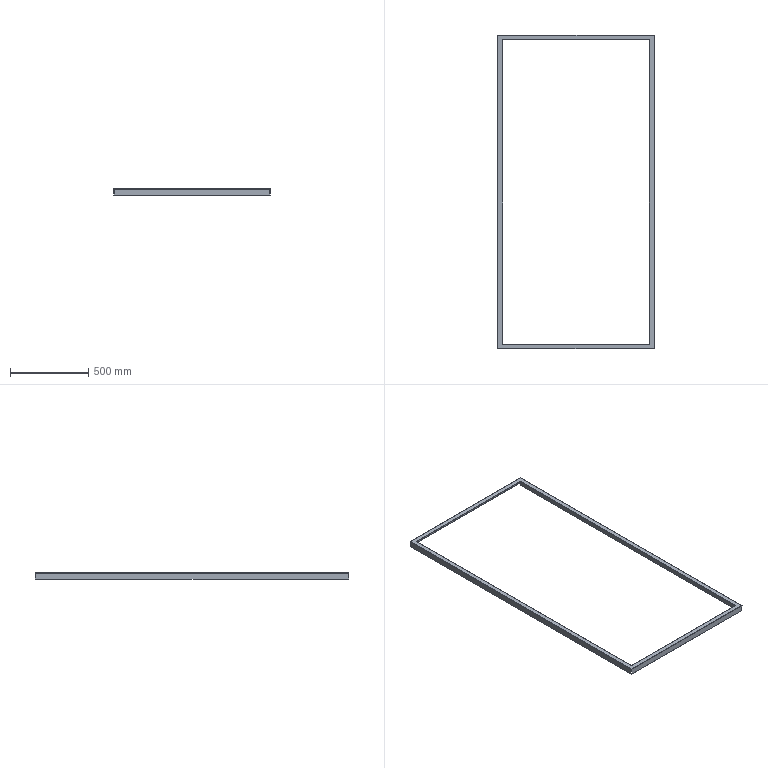Part | SolidWorks | features EdgeFlange 2, FlatPattern 1, ICE 1, SMBaseFlange 1, SheetMetal 1 | 1 solid | 74 faces | box 1000 x 2000 x 40 mm | volume 1030589 mm3 | plane 54 | cylinder 12 | spline 8 | commonest cylinder face diameters 0.2 x6 4.2 x6